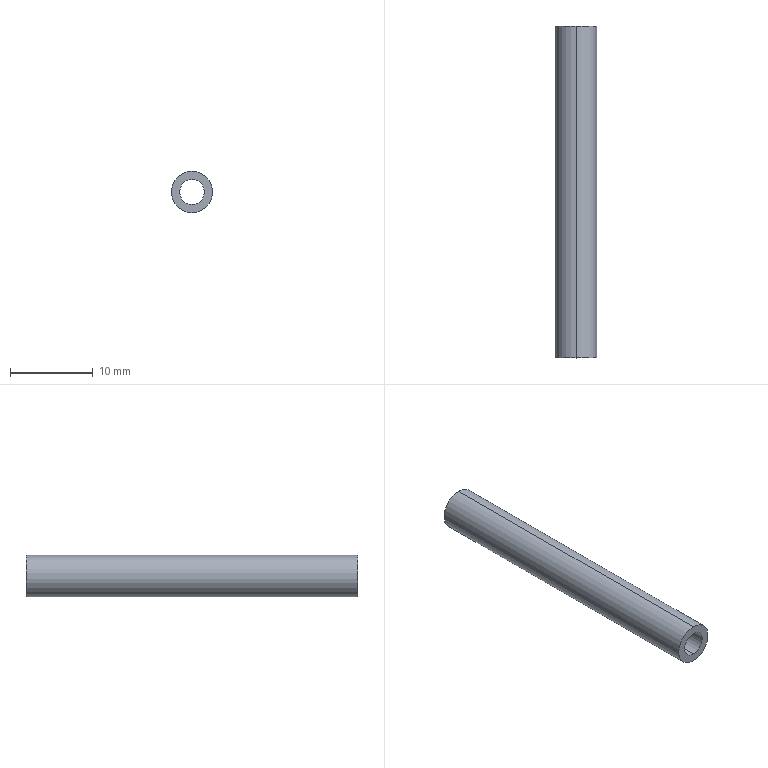Part | SolidWorks | features Extrusion 1 | 1 solid | 6 faces | box 5 x 40 x 5 mm | volume 502.655 mm3 | cylinder 4 | plane 2 | commonest cylinder face diameters 3 x2 5 x2
STEP:
#1=CARTESIAN_POINT('',(0.,40.,-1.5));
#2=VERTEX_POINT('',#1);
#3=CARTESIAN_POINT('',(0.,40.,1.5));
#4=VERTEX_POINT('',#3);
#5=CARTESIAN_POINT('',(0.,40.,0.));
#6=DIRECTION('',(0.,1.,0.));
#7=DIRECTION('',(0.,0.,1.));
#8=AXIS2_PLACEMENT_3D('',#5,#6,#7);
#9=CIRCLE('',#8,1.5);
#10=EDGE_CURVE('',#2,#4,#9,.T.);
#11=ORIENTED_EDGE('',*,*,#10,.T.);
#12=CARTESIAN_POINT('',(0.,0.,1.5));
#13=VERTEX_POINT('',#12);
#14=CARTESIAN_POINT('',(0.,40.,1.5));
#15=DIRECTION('',(0.,-1.,0.));
#16=VECTOR('',#15,1000.);
#17=LINE('',#14,#16);
#18=EDGE_CURVE('',#4,#13,#17,.T.);
#19=ORIENTED_EDGE('',*,*,#18,.T.);
#20=CARTESIAN_POINT('',(0.,0.,-1.5));
#21=VERTEX_POINT('',#20);
#22=CARTESIAN_POINT('',(0.,0.,0.));
#23=DIRECTION('',(0.,1.,0.));
#24=DIRECTION('',(0.,0.,1.));
#25=AXIS2_PLACEMENT_3D('',#22,#23,#24);
#26=CIRCLE('',#25,1.5);
#27=EDGE_CURVE('',#21,#13,#26,.T.);
#28=ORIENTED_EDGE('',*,*,#27,.F.);
#29=CARTESIAN_POINT('',(0.,40.,-1.5));
#30=DIRECTION('',(0.,-1.,0.));
#31=VECTOR('',#30,1000.);
#32=LINE('',#29,#31);
#33=EDGE_CURVE('',#2,#21,#32,.T.);
#34=ORIENTED_EDGE('',*,*,#33,.F.);
#35=EDGE_LOOP('',(#11,#19,#28,#34));
#36=FACE_OUTER_BOUND('',#35,.T.);
#37=CARTESIAN_POINT('',(0.,40.,0.));
#38=DIRECTION('',(0.,-1.,0.));
#39=DIRECTION('',(0.,0.,-1.));
#40=AXIS2_PLACEMENT_3D('',#37,#38,#39);
#41=CYLINDRICAL_SURFACE('',#40,1.5);
#42=ADVANCED_FACE('',(#36),#41,.F.);
#43=CARTESIAN_POINT('',(0.,40.,2.5));
#44=VERTEX_POINT('',#43);
#45=CARTESIAN_POINT('',(0.,40.,-2.5));
#46=VERTEX_POINT('',#45);
#47=CARTESIAN_POINT('',(0.,40.,0.));
#48=DIRECTION('',(0.,1.,0.));
#49=DIRECTION('',(0.,0.,1.));
#50=AXIS2_PLACEMENT_3D('',#47,#48,#49);
#51=CIRCLE('',#50,2.5);
#52=EDGE_CURVE('',#44,#46,#51,.T.);
#53=ORIENTED_EDGE('',*,*,#52,.F.);
#54=CARTESIAN_POINT('',(0.,0.,2.5));
#55=VERTEX_POINT('',#54);
#56=CARTESIAN_POINT('',(0.,40.,2.5));
#57=DIRECTION('',(0.,-1.,0.));
#58=VECTOR('',#57,1000.);
#59=LINE('',#56,#58);
#60=EDGE_CURVE('',#44,#55,#59,.T.);
#61=ORIENTED_EDGE('',*,*,#60,.T.);
#62=CARTESIAN_POINT('',(0.,0.,-2.5));
#63=VERTEX_POINT('',#62);
#64=CARTESIAN_POINT('',(0.,0.,0.));
#65=DIRECTION('',(0.,1.,0.));
#66=DIRECTION('',(0.,0.,1.));
#67=AXIS2_PLACEMENT_3D('',#64,#65,#66);
#68=CIRCLE('',#67,2.5);
#69=EDGE_CURVE('',#55,#63,#68,.T.);
#70=ORIENTED_EDGE('',*,*,#69,.T.);
#71=CARTESIAN_POINT('',(0.,40.,-2.5));
#72=DIRECTION('',(0.,-1.,0.));
#73=VECTOR('',#72,1000.);
#74=LINE('',#71,#73);
#75=EDGE_CURVE('',#46,#63,#74,.T.);
#76=ORIENTED_EDGE('',*,*,#75,.F.);
#77=EDGE_LOOP('',(#53,#61,#70,#76));
#78=FACE_OUTER_BOUND('',#77,.T.);
#79=CARTESIAN_POINT('',(0.,40.,0.));
#80=DIRECTION('',(0.,-1.,0.));
#81=DIRECTION('',(0.,0.,-1.));
#82=AXIS2_PLACEMENT_3D('',#79,#80,#81);
#83=CYLINDRICAL_SURFACE('',#82,2.5);
#84=ADVANCED_FACE('',(#78),#83,.T.);
#85=CARTESIAN_POINT('',(0.,40.,0.));
#86=DIRECTION('',(0.,1.,0.));
#87=DIRECTION('',(0.,0.,1.));
#88=AXIS2_PLACEMENT_3D('',#85,#86,#87);
#89=CIRCLE('',#88,2.5);
#90=EDGE_CURVE('',#46,#44,#89,.T.);
#91=ORIENTED_EDGE('',*,*,#90,.T.);
#92=ORIENTED_EDGE('',*,*,#52,.T.);
#93=EDGE_LOOP('',(#91,#92));
#94=FACE_OUTER_BOUND('',#93,.T.);
#95=ORIENTED_EDGE('',*,*,#10,.F.);
#96=CARTESIAN_POINT('',(0.,40.,0.));
#97=DIRECTION('',(0.,1.,0.));
#98=DIRECTION('',(0.,0.,1.));
#99=AXIS2_PLACEMENT_3D('',#96,#97,#98);
#100=CIRCLE('',#99,1.5);
#101=EDGE_CURVE('',#4,#2,#100,.T.);
#102=ORIENTED_EDGE('',*,*,#101,.F.);
#103=EDGE_LOOP('',(#95,#102));
#104=FACE_BOUND('',#103,.T.);
#105=CARTESIAN_POINT('',(0.,40.,0.));
#106=DIRECTION('',(0.,1.,0.));
#107=DIRECTION('',(0.,0.,1.));
#108=AXIS2_PLACEMENT_3D('',#105,#106,#107);
#109=PLANE('',#108);
#110=ADVANCED_FACE('',(#94,#104),#109,.T.);
#111=CARTESIAN_POINT('',(0.,0.,0.));
#112=DIRECTION('',(0.,1.,0.));
#113=DIRECTION('',(0.,0.,1.));
#114=AXIS2_PLACEMENT_3D('',#111,#112,#113);
#115=CIRCLE('',#114,2.5);
#116=EDGE_CURVE('',#63,#55,#115,.T.);
#117=ORIENTED_EDGE('',*,*,#116,.F.);
#118=ORIENTED_EDGE('',*,*,#69,.F.);
#119=EDGE_LOOP('',(#117,#118));
#120=FACE_OUTER_BOUND('',#119,.T.);
#121=ORIENTED_EDGE('',*,*,#27,.T.);
#122=CARTESIAN_POINT('',(0.,0.,0.));
#123=DIRECTION('',(0.,1.,0.));
#124=DIRECTION('',(0.,0.,1.));
#125=AXIS2_PLACEMENT_3D('',#122,#123,#124);
#126=CIRCLE('',#125,1.5);
#127=EDGE_CURVE('',#13,#21,#126,.T.);
#128=ORIENTED_EDGE('',*,*,#127,.T.);
#129=EDGE_LOOP('',(#121,#128));
#130=FACE_BOUND('',#129,.T.);
#131=CARTESIAN_POINT('',(0.,0.,0.));
#132=DIRECTION('',(0.,1.,0.));
#133=DIRECTION('',(0.,0.,1.));
#134=AXIS2_PLACEMENT_3D('',#131,#132,#133);
#135=PLANE('',#134);
#136=ADVANCED_FACE('',(#120,#130),#135,.F.);
#137=ORIENTED_EDGE('',*,*,#60,.F.);
#138=ORIENTED_EDGE('',*,*,#90,.F.);
#139=ORIENTED_EDGE('',*,*,#75,.T.);
#140=ORIENTED_EDGE('',*,*,#116,.T.);
#141=EDGE_LOOP('',(#137,#138,#139,#140));
#142=FACE_OUTER_BOUND('',#141,.T.);
#143=CARTESIAN_POINT('',(0.,40.,0.));
#144=DIRECTION('',(0.,-1.,0.));
#145=DIRECTION('',(0.,0.,-1.));
#146=AXIS2_PLACEMENT_3D('',#143,#144,#145);
#147=CYLINDRICAL_SURFACE('',#146,2.5);
#148=ADVANCED_FACE('',(#142),#147,.T.);
#149=ORIENTED_EDGE('',*,*,#18,.F.);
#150=ORIENTED_EDGE('',*,*,#101,.T.);
#151=ORIENTED_EDGE('',*,*,#33,.T.);
#152=ORIENTED_EDGE('',*,*,#127,.F.);
#153=EDGE_LOOP('',(#149,#150,#151,#152));
#154=FACE_OUTER_BOUND('',#153,.T.);
#155=CARTESIAN_POINT('',(0.,40.,0.));
#156=DIRECTION('',(0.,-1.,0.));
#157=DIRECTION('',(0.,0.,-1.));
#158=AXIS2_PLACEMENT_3D('',#155,#156,#157);
#159=CYLINDRICAL_SURFACE('',#158,1.5);
#160=ADVANCED_FACE('',(#154),#159,.F.);
#161=CLOSED_SHELL('',(#42,#84,#110,#136,#148,#160));
#162=MANIFOLD_SOLID_BREP('',#161);
#163=CARTESIAN_POINT('',(0.,0.,0.));
#164=DIRECTION('',(0.,0.,1.));
#165=DIRECTION('',(1.,0.,0.));
#166=AXIS2_PLACEMENT_3D('',#163,#164,#165);
#167=(LENGTH_UNIT()NAMED_UNIT(*)SI_UNIT(.MILLI.,.METRE.));
#168=UNCERTAINTY_MEASURE_WITH_UNIT(LENGTH_MEASURE(0.00001),#167,'','');
#169=(NAMED_UNIT(*)PLANE_ANGLE_UNIT()SI_UNIT($,.RADIAN.));
#170=(NAMED_UNIT(*)SI_UNIT($,.STERADIAN.)SOLID_ANGLE_UNIT());
#171=(GEOMETRIC_REPRESENTATION_CONTEXT(3)GLOBAL_UNCERTAINTY_ASSIGNED_CONTEXT((#168))GLOBAL_UNIT_ASSIGNED_CONTEXT((#167,#169,#170))REPRESENTATION_CONTEXT('',''));
#172=ADVANCED_BREP_SHAPE_REPRESENTATION('',(#162,#166),#171);